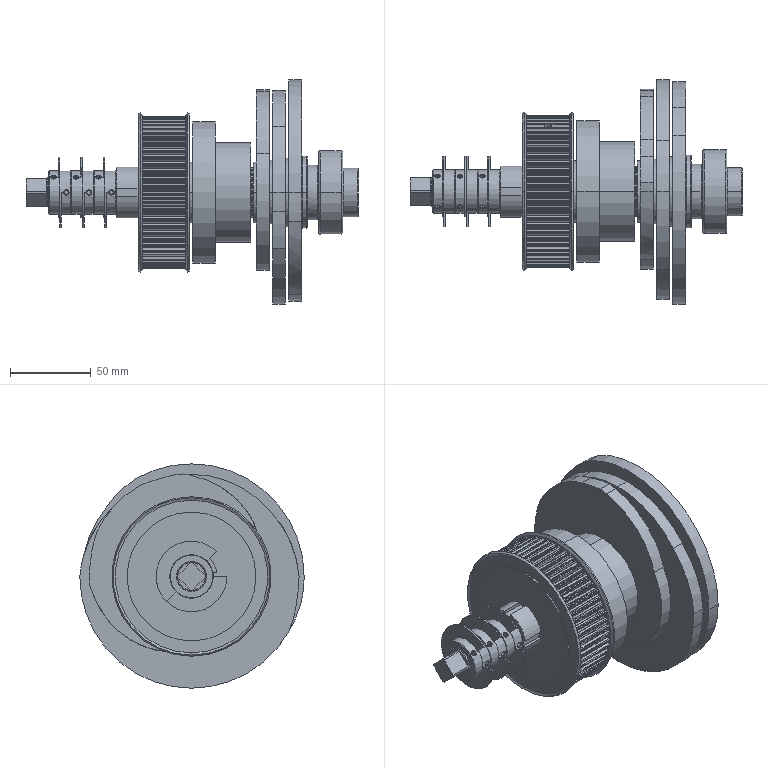Part | NX | 21 solids | 1106 faces | box 206 x 139.21 x 139.21 mm | volume 763016 mm3 | cylinder 738 | plane 221 | cone 94 | spline 29 | torus 24 | commonest cylinder face diameters 0.5 x124 1.1 x124 6.55 x124 94.53 x88 90.99 x63 2.5 x24